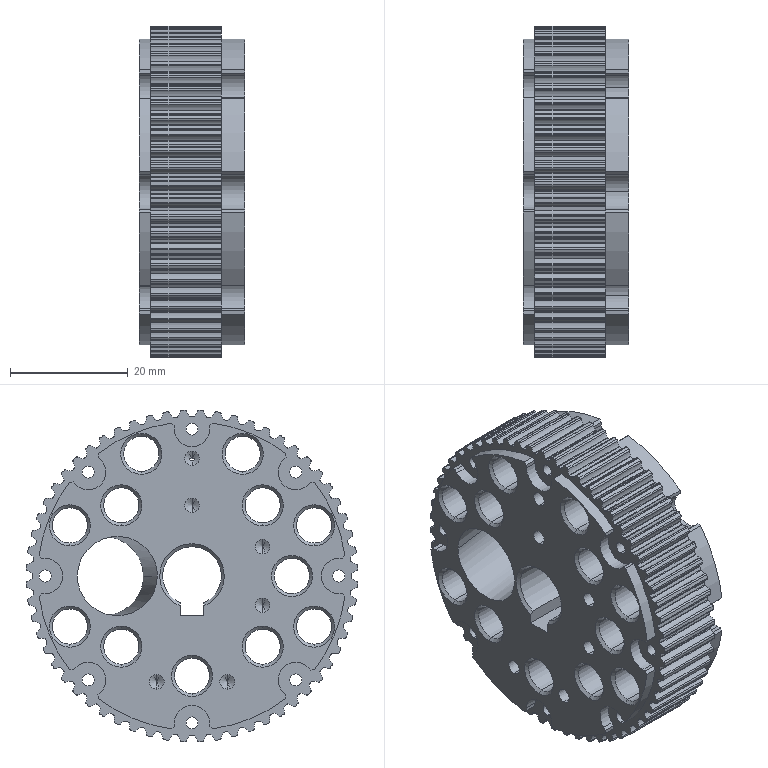Part | SolidWorks | features ICE 11, Chamfer 5, HoleWzd 5, CirPattern 3, BaseBody 1, RevCut 1 | 1 solid | 776 faces | box 18 x 56.48 x 56.48 mm | volume 29168 mm3 | cylinder 633 | plane 74 | cone 69 | commonest cylinder face diameters 0.56 x146 0.3 x136 3.95 x130 54.31 x61 56.53 x60 6 x52